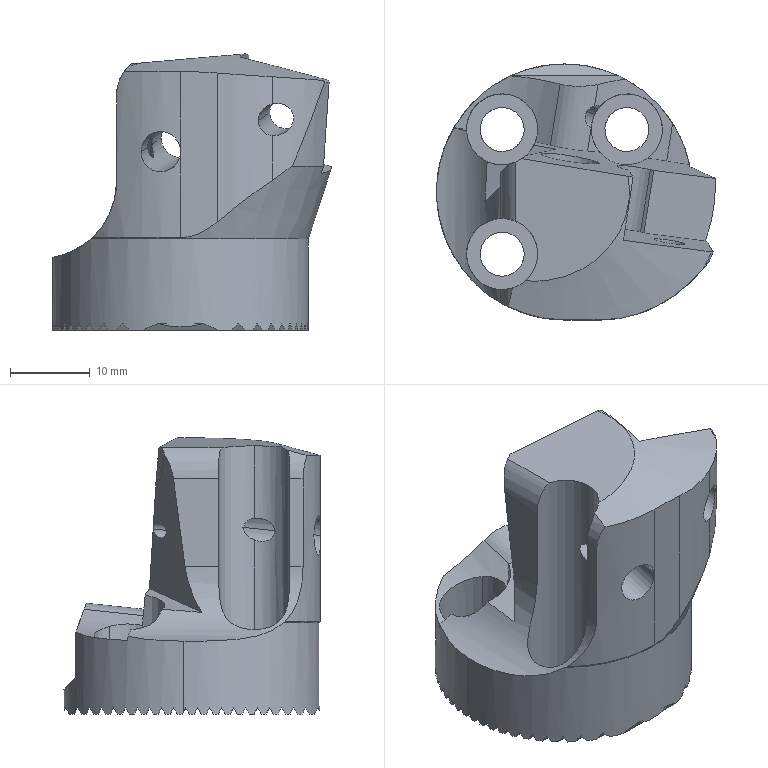NC program | Mastercam | posted with a generic post
Lines 1 to 700 of 7888:
%
:0001()
(MATERIAL - ALUMINUM MM - 2024)
(T4|12 FEMR |H4|XY STOCK TO LEAVE - .15|Z STOCK TO LEAVE - 0.)
(T5|6 FEMR |H5|XY STOCK TO LEAVE - .1|Z STOCK TO LEAVE - .1)
(T6|4 FEMR |H6|D6|WEAR COMP|TOOL DIA. - 4.|XY STOCK TO LEAVE - .05|Z STOCK TO LEAVE - .1)
(T7|4 FEMF |H7|D7|WEAR COMP|TOOL DIA. - 4.|XY STOCK TO LEAVE - 0.|Z STOCK TO LEAVE - .02)
(T9|12 FEMF |H9|D9|WEAR COMP|TOOL DIA. - 12.)
(T10|30 BNOS |H10|D10|WEAR COMP|TOOL DIA. - 30.)
(T12|6 SPD |H12)
(T3|4.3 DR |H3)
(T13|3.3 DR |H13)
(T1|2 DR |H1)
(T11|4 FEM |H11)
(T18|5.5 FL |H18)
(T14|3.15 THML |H14|D14|WEAR COMP|TOOL DIA. - 3.15)
(T16|M5 X 0.8 RH |H16)
(T15|2.5 BM |H15)
(T2|6 120DSPD |H2)
(T17|3 DR |H17)
N100 G21
N102 G0 G17 G40 G80 G90 G94 G98
N104 G0 G28 G91 Z0.
N106 G0 G28 X0. Y0.
(12 FEMR |TOOL - 4|DIA. OFF. - 4|LEN. - 4|TOOL DIA. - 12.)
N108 T4 M6
N110 G0 G54 G90 X25.327 Y-16.016 C0. B0. S3500 M3
N112 G43 H4 Z84.532
N114 Z36.532
N116 G1 Z9.782 F2000.
N118 X24.063 Y-14.854 Z9.631 F2500.
N120 G3 X23.099 Y-14.284 Z9.532 I-1.827 J-1.988
N122 X22.513 Y-14.091 I-2.505 J-6.624
N124 X22.076 Y-14.542 I1.447 J-1.839
N126 X20.527 Y-16.382 I63.197 J-54.78
N128 G2 X15.136 Y-21.366 I-22.56 J18.993
N130 X4.096 Y-25.849 I-15.051 J21.233
N132 X1.821 Y-25.988 I-2.275 J18.516
N134 X-.909 Y-25.787 J18.655
N136 X-14.128 Y-19.713 I3.68 J25.432
N138 X-21.534 Y-8.928 I17.053 J19.644
N140 G1 X-21.941
N142 X-22.348
N144 G3 X-23.443 Y-9.16 Z9.606 J-2.7
N146 G1 X-25.013 Y-9.857 Z9.72
N148 G3 X-25.778 Y-10.368 Z9.782 I1.096 J-2.467
N150 X-26.617 Y-12.324 I1.861 J-1.956
N152 X-24.238 Y-15.005 I2.7
N154 G2 X-19.964 Y-15.517 I-24.723 J-224.737 F9500.
N156 X-18.544 Y-16.345 I-.297 J-2.139
N158 G3 X-4.251 Y-26.044 I21.482 J16.278
N160 X2.015 Y-26.912 I6.266 J22.19
N162 X2.462 Y-26.907 J23.058
N164 X6.706 Y-26.267 I-.54 J17.966
N166 X17.663 Y-20.587 I-6.831 J26.583
N168 G2 X18.923 Y-20.181 I1.26 J-1.754
N170 X19.179 Y-20.196 J-2.16
N172 G1 X23.134 Y-20.669
N174 G3 X23.454 Y-20.688 I.32 J2.681
N176 X26.154 Y-17.988 J2.7
N178 X25.843 Y-16.729 I-2.7
N180 X25.281 Y-16. Z9.72 I-2.389 J-1.259 F2500.
N182 G1 X24.017 Y-14.838 Z9.606
N184 G3 X23.053 Y-14.268 Z9.532 I-1.827 J-1.988
N186 X22.433 Y-14.074 I-1.233 J-2.856
N188 X21.719 Y-14.71 I2.987 J-4.073
N190 X19.861 Y-16.692 I53.778 J-52.268
N192 G2 X15.195 Y-20.861 I-23.789 J21.932
N194 X5.469 Y-25.196 I-15.123 J20.849
N196 X1.763 Y-25.549 I-3.706 J19.282
N198 X-1.087 Y-25.341 J19.635
N200 X-11.914 Y-20.963 I3.638 J24.572
N202 X-20.634 Y-10.181 I14.952 J21.008
N204 G3 X-21.069 Y-9.298 I-25.07 J-11.815
N206 X-21.342 Y-8.928 I-1.084 J-.514
N208 G1 X-21.749
N210 G3 X-22.845 Y-9.16 Z9.606 J-2.7
N212 G1 X-24.414 Y-9.857 Z9.72
N214 G3 X-25.179 Y-10.368 Z9.782 I1.095 J-2.467
N216 X-26.018 Y-12.324 I1.86 J-1.956 F9500.
N218 X-23.642 Y-15.005 I2.699
N220 G2 X-19.481 Y-15.507 I-24.132 J-217.33
N222 X-18.075 Y-16.322 I-.3 J-2.14
N224 G3 X-3.802 Y-25.748 I20.927 J16.168
N226 X1.808 Y-26.475 I5.61 J21.278
N228 X3.413 Y-26.416 J22.005
N230 X8.741 Y-25.253 I-1.778 J20.92
N232 X17.208 Y-20.488 I-9.096 J26.07
N234 G2 X18.445 Y-20.099 I1.237 J-1.771
N236 X18.704 Y-20.114 J-2.16
N238 G1 X23.036 Y-20.637
N240 G3 X23.36 Y-20.657 I.324 J2.68
N242 X26.06 Y-17.957 J2.7
N244 X25.748 Y-16.697 I-2.7
N246 X25.187 Y-15.968 Z9.72 I-2.388 J-1.26 F2500.
N248 G1 X23.922 Y-14.807 Z9.606
N250 G3 X22.959 Y-14.236 Z9.532 I-1.827 J-1.988
N252 X22.374 Y-14.066 I-1.101 J-2.683
N254 X22.313 Y-14.06 I-.144 J-1.191
N256 X21.573 Y-14.633 I2.623 J-4.149
N258 X19.45 Y-16.705 I41.164 J-44.288
N260 G2 X15.167 Y-20.423 I-25.523 J25.078
N262 X6.987 Y-24.419 I-15.258 J20.865
N264 X1.726 Y-25.122 I-5.261 J19.345
N266 X-1.631 Y-24.838 J20.048
N268 X-12.379 Y-20.136 I4.116 J24.041
N270 X-19.695 Y-11.291 I15.466 J20.24
N272 G3 X-20.718 Y-9.43 I-20.626 J-10.132
N274 X-21.323 Y-8.928 I-1.027 J-.621
N276 G1 X-21.556 Y-9.857 Z9.595
N278 G3 X-21.752 Y-11.447 Z9.702 I6.34 J-1.59
N280 X-21.642 Y-12.646 Z9.782 I6.536
N282 X-18.925 Y-16.829 I6.426 J1.199 F9500.
N284 G1 X-7.24 Y-24.879
N286 G3 X-5.367 Y-25.77 I3.708 J5.382
N288 X1.244 Y-26.717 I6.611 J22.596
N290 X13.879 Y-23.04 J23.543
N292 G1 X24.283 Y-16.423
N294 X25.063 Y-15.927 Z9.72 F2500.
N296 X23.798 Y-14.765 Z9.606
N298 G3 X22.834 Y-14.194 Z9.532 I-1.827 J-1.988
N300 X22.21 Y-14.058 I-.624 J-1.364
N302 X22.151 Y-14.06 J-1.5
N304 X21.17 Y-14.768 I2.987 J-5.17
N306 X18.98 Y-16.767 I38.187 J-44.029
N308 G2 X14.652 Y-20.34 I-26.402 J27.573
N310 X7.861 Y-23.741 I-14.905 J21.276
N312 X1.707 Y-24.696 I-6.154 J19.347
N314 X-2.293 Y-24.299 J20.302
N316 X-13.296 Y-18.888 I4.768 J23.585
N318 X-18.729 Y-12.278 I16.488 J19.093
N320 G3 X-20.042 Y-10.033 I-75.514 J-42.648
N322 X-20.484 Y-9.389 I-27.464 J-18.386
N324 X-21.11 Y-8.928 I-.987 J-.683
N326 G1 X-21.305 Y-9.857 Z9.595
N328 G3 X-21.44 Y-11.156 Z9.682 I6.166 J-1.299
N330 X-21.26 Y-12.653 Z9.782 I6.301
N332 X-18.83 Y-16.264 I6.121 J1.497 F9500.
N334 G1 X-7.75 Y-24.269
N336 G3 X-6.03 Y-25.147 I3.69 J5.108
N338 X1.57 Y-26.366 I7.6 J23.09
N340 X13.907 Y-23.002 J24.309
N342 G1 X24.732 Y-16.625
N344 X24.828 Y-16.569 Z9.774 F2500.
N346 G3 X25.043 Y-16.193 Z9.744 I-.221 J.376
N348 X24.902 Y-15.872 Z9.72 I-.436
N350 G1 X23.638 Y-14.711 Z9.606
N352 G3 X22.674 Y-14.14 Z9.532 I-1.827 J-1.988
N354 X22.232 Y-14.057 I-.442 J-1.136
N356 X21.896 Y-14.104 J-1.219
N358 X21.255 Y-14.545 I1.025 J-2.182
N360 G2 X17.18 Y-18.101 I-18.947 J17.598
N362 G3 X16.536 Y-18.58 I237.78 J-319.951
N364 G2 X12.22 Y-21.428 I-22.586 J29.54
N366 X6.428 Y-23.721 I-11.391 J20.308
N368 X1.693 Y-24.279 I-4.735 J19.815
N370 X-3.706 Y-23.55 J20.373
N372 X-15.397 Y-16.261 I6.303 J23.129
N374 X-16.881 Y-14.418 I20.422 J17.958
N376 X-19.755 Y-10.15 I17.443 J14.849
N378 G3 X-20.293 Y-9.363 I-6.125 J-3.611
N380 X-20.812 Y-8.962 I-.966 J-.712
N382 X-21.095 Y-8.928 I-.283 J-1.166
N384 X-23.066 Y-9.783 Z9.678 J-2.7
N386 G1 X-23.649 Y-10.406 Z9.735
N388 G3 X-24.059 Y-10.979 Z9.782 I1.971 J-1.845
N390 X-24.377 Y-12.251 I2.381 J-1.272 F9500.
N392 X-21.678 Y-14.95 I2.699
N394 X-19.961 Y-14.335 J2.699
N396 X-18.978 Y-12.251 Z9.624 I-1.717 J2.084 F2500.
N398 X-19.327 Y-10.922 Z9.532 I-2.7
N400 G2 X-20.048 Y-9.556 I19.393 J11.113
N402 G3 X-20.789 Y-8.971 I-1.081 J-.607
N404 X-21.11 Y-8.927 Z9.553 I-.321 J-1.157
N406 X-22.169 Y-9.563 Z9.639 J-1.201
N408 G1 X-22.503 Y-10.189 Z9.686
N410 G3 X-22.689 Y-10.931 Z9.738 I1.39 J-.742
N412 X-22.55 Y-11.577 Z9.782 I1.576
N414 X-21.646 Y-12.413 I1.437 J.646 F9500.
N416 X-21.113 Y-12.506 Z9.746 I.533 J1.482 F2500.
N418 X-19.538 Y-10.931 Z9.582 J1.575
N420 X-19.715 Y-10.207 Z9.532 I-1.575
N422 G2 X-20.013 Y-9.608 I19.715 J10.207
N424 G3 X-21.095 Y-8.928 I-1.082 J-.52
N426 X-22.19 Y-9.16 Z9.606 J-2.7
N428 G1 X-23.76 Y-9.857 Z9.72
N430 G3 X-24.525 Y-10.368 Z9.782 I1.096 J-2.467
N432 X-25.364 Y-12.324 I1.861 J-1.956 F9500.
N434 X-23.093 Y-14.99 I2.7
N436 G1 X-17.635 Y-15.868
N438 G2 X-16.345 Y-16.586 I-.342 J-2.132
N440 G3 X-3.918 Y-24.455 I18.925 J16.14
N442 X1.691 Y-25.206 I5.609 J20.576
N444 X7.761 Y-24.324 J21.327
N446 X14.009 Y-21.457 I-7.621 J24.852
N448 G2 X15.106 Y-21.158 I1.097 J-1.861
N450 X15.448 Y-21.185 J-2.16
N452 G1 X20.574 Y-22.009
N454 G3 X21.002 Y-22.043 I.428 J2.666
N456 X23.702 Y-19.343 J2.7
N458 X21.574 Y-16.704 I-2.7
N460 X21.002 Y-16.643 Z9.744 I-.572 J-2.639 F2500.
N462 X20.386 Y-16.714 Z9.702 J-2.7
N464 G1 X20.385
N466 X18.98 Y-17.044 Z9.606
N468 G3 X17.966 Y-17.52 Z9.532 I.617 J-2.629
N470 G2 X14.756 Y-19.601 I-16.018 J21.202
N472 X11.208 Y-21.561 I-26.515 J43.803
N474 X5.266 Y-23.543 I-10.01 J20.109
N476 X1.705 Y-23.853 I-3.561 J20.299
N478 X-4.833 Y-22.789 J20.609
N480 X-13.656 Y-17.503 I7.425 J22.401
N482 X-17.147 Y-14.101 I13.656 J17.503
N484 G3 X-18.022 Y-13.402 Z9.606 I-2.085 J-1.715
N486 G1 X-19.285 Y-12.769 Z9.7
N488 G3 X-19.883 Y-12.628 Z9.741 I-.598 J-1.193
N490 X-20.471 Y-12.764 Z9.782 J-1.334
N492 X-21.107 Y-13.428 I.588 J-1.198 F9500.
N494 G1 X-22.287 Y-16.133
N496 G3 X-22.398 Y-16.667 I1.224 J-.534
N498 X-21.614 Y-17.883 I1.335
N500 G1 X-14.889 Y-20.925
N502 G3 X6.013 Y-25.433 I20.902 J46.199
N504 X14.41 Y-24.733 J50.707
N506 G1 X19.513 Y-23.877
N508 G3 X21.779 Y-21.199 I-.449 J2.678
N510 X19.291 Y-18.493 I-2.715
N512 X19.064 Y-18.483 Z9.767 I-.227 J-2.706 F2500.
N514 X18.743 Y-18.503 Z9.745 J-2.716
N516 G1 X18.098 Y-18.579 Z9.702
N518 X16.664 Y-18.75 Z9.606
N520 G3 X15.604 Y-19.11 Z9.532 I.319 J-2.681
N522 G2 X12.148 Y-20.826 I-13.308 J22.47
N524 X8.231 Y-22.392 I-15.934 J34.155
N526 X1.744 Y-23.434 I-6.487 J19.662
N528 X-5.935 Y-21.958 J20.704
N530 X-10.399 Y-19.614 I8.614 J21.825
N532 X-14.116 Y-17.134 I10.399 J19.614
N534 G3 X-15.11 Y-16.616 Z9.606 I-1.717 J-2.084
N536 G1 X-16.471 Y-16.238 Z9.7
N538 G3 X-16.829 Y-16.189 Z9.724 I-.358 J-1.287
N540 X-17.636 Y-16.46 Z9.782 J-1.336
N542 X-18.061 Y-17.008 I.807 J-1.065 F9500.
N544 G1 X-19.203 Y-19.731
N546 G3 X-19.307 Y-20.248 I1.233 J-.517
N548 X-18.313 Y-21.539 I1.337
N550 X12.208 Y-25.517 I30.521 J115.1
N552 X17.041 Y-25.419 J119.078
N554 X19.638 Y-22.714 I-.11 J2.705
N556 X17.119 Y-20.013 I-2.707
N558 X16.931 Y-20.006 Z9.769 I-.188 J-2.701 F2500.
N560 G1 X16.9 Y-20.007 Z9.767
N562 X15.891 Y-20.019 Z9.7
N564 X14.477 Y-20.035 Z9.606
N566 G3 X13.385 Y-20.28 Z9.532 I.032 J-2.7
N568 G2 X10.176 Y-21.457 I-9.354 J20.546
N570 X6.628 Y-22.471 I-12.999 J38.767
N572 X1.85 Y-23.021 I-4.778 J20.468
N574 X-6.993 Y-21.07 J21.018
N576 X-10.717 Y-19.442 I6.993 J21.07
N578 G3 X-12.02 Y-19.107 Z9.622 I-1.303 J-2.365
N580 X-14.122 Y-20.113 Z9.782 J-2.7
N582 X-14.72 Y-21.807 I2.102 J-1.694 F9500.
N584 X-12.236 Y-24.498 I2.7
N586 G1 X11.728 Y-26.426
N588 G3 X11.945 Y-26.435 I.217 J2.692
N590 X14.646 Y-23.734 J2.701
N592 X14.329 Y-22.467 I-2.701
N594 X11.945 Y-21.034 Z9.588 I-2.384 J-1.267 F2500.
N596 X11.111 Y-21.166 Z9.532 J-2.7
N598 G2 X7.78 Y-21.965 I-6.85 J21.232
N600 X4.086 Y-22.527 I-7.479 J36.716
N602 X2.041 Y-22.624 I-2.045 J21.433
N604 X-3.282 Y-21.956 J21.53
N606 X-7.613 Y-20.854 I3.282 J21.956
N608 G3 X-8.539 Y-20.69 Z9.595 I-.926 J-2.536
N610 X-10.876 Y-22.038 Z9.782 J-2.7
N612 X-11.239 Y-23.39 I2.337 J-1.352 F9500.
N614 X-8.696 Y-26.086 I2.7
N616 G1 X9.125 Y-27.127
N618 G3 X9.282 Y-27.132 I.157 J2.695
N620 X11.982 Y-24.432 J2.7
N622 X11.797 Y-23.448 I-2.7
N624 X9.282 Y-21.731 Z9.568 I-2.515 J-.984 F2500.
N626 X8.75 Y-21.785 Z9.532 J-2.701
N628 G2 X4.925 Y-22.206 I-4.342 J21.859
N630 X2.83 Y-22.274 I-2.095 J32.189
N632 X.646 Y-22.2 J32.257
N634 G1 X.239
N636 G2 X.021 Y-22.201 I-.218 J22.375
N638 X-3.646 Y-21.899 J22.376
N640 G3 X-4.09 Y-21.862 Z9.562 I-.444 J-2.663
N642 X-6.635 Y-23.663 Z9.782 J-2.7
N644 X-6.789 Y-24.562 I2.545 J-.899 F9500.
N646 X-4.166 Y-27.261 I2.699
N648 G1 X6.023 Y-27.55
N650 G3 X6.1 Y-27.551 I.077 J2.698
N652 X8.799 Y-24.852 J2.699
N654 X8.723 Y-24.214 I-2.699
N656 X6.1 Y-22.153 Z9.543 I-2.623 J-.638 F2500.
N658 X5.928 Y-22.157 Z9.532 J-2.699
N660 G2 X4.074 Y-22.208 I-1.854 J33.96
N662 X3.359 Y-22.2 J34.011
N664 G1 X2.952
N666 X0.
N668 G3 X-1.096 Y-22.432 Z9.606 J-2.7
N670 G1 X-2.387 Y-23.006 Z9.7
N672 G3 X-3.36 Y-23.738 Z9.782 I1.096 J-2.467
N674 X-3.991 Y-25.473 I2.069 J-1.735 F9500.
N676 X-1.291 Y-28.173 I2.7
N678 X-.435 Y-28.034 J2.7
N680 G1 X23.234 Y-20.118
N682 G3 X25.077 Y-17.558 I-.856 J2.56
N684 G1 X25.063 Y-17.283
N686 X25.021 Y-17.011
N688 X24.952 Y-16.744
N690 G3 X24.312 Y-15.673 Z9.698 I-2.575 J-.814 F2500.
N692 G1 X23.089 Y-14.419 Z9.582
N694 G3 X22.428 Y-14.073 Z9.532 I-.859 J-.838
N696 X22.23 Y-14.057 I-.198 J-1.184
N698 X21.346 Y-14.446 J-1.2
N700 G2 X20.786 Y-15.036 I-18.731 J17.193
N702 G3 X20.186 Y-15.982 Z9.641 I1.93 J-1.889
N704 G1 X19.682 Y-17.335 Z9.782
N706 G0 Z84.532
N708 C9. B-84.
N710 X13.169 Y27.825
N712 Z56.789
N714 Z8.789
N716 G1 Z7.039 F2000.
N718 X12.949 Y26.122 Z6.888 F2500.
N720 G3 X12.927 Y25.777 Z6.858 I2.678 J-.345
N722 X13.04 Y25.006 Z6.789 I2.7
N724 G1 X13.214 Y24.421
N726 X13.479 Y24.43
N728 G3 X15.936 Y24.972 I-3.086 J19.807
N730 X19.38 Y25.938 I-41.706 J155.352
N732 G2 X22.887 Y26.414 I4.411 J-19.32
N734 X27.937 Y26.532 I5.05 J-108.202
N736 X28.468 Y26.531 J-108.32
N738 X30.923 Y26.536 I3.173 J-965.361
N740 G1 X31.331
N742 X34.477
N744 G2 X37.69 Y25.537 I-.189 J-6.275
N746 X40.163 Y22.946 I-4.167 J-6.454
N748 X41.389 Y19.73 I-9.311 J-5.391
N750 X41.824 Y16.067 I-21.737 J-4.435
N752 X41.922 Y10.577 I-154.13 J-5.49
N754 X41.919 Y9.72 I-154.228
N756 G1 X41.92 Y9.311
N758 X41.913 Y-16.351
N760 G2 X40.808 Y-19.535 I-6.329 J.413
N762 X38.186 Y-21.918 I-6.343 J4.345
N764 X34.999 Y-23.084 I-5.317 J9.594
N766 X31.365 Y-23.498 I-4.394 J22.434
N768 X25.885 Y-23.592 I-5.48 J160.417
N770 X25.027 Y-23.589 J160.511
N772 G1 X24.618
N774 X15.311 Y-23.592
N776 Y-24.406
N778 G3 X15.543 Y-25.502 Z6.863 I2.7
N780 G1 X16.24 Y-27.071 Z6.977
N782 G3 X16.692 Y-27.877 Z7.039 I4.547 J2.019
N784 X20.787 Y-30.027 I4.095 J2.825
N786 X22.619 Y-29.678 J4.975
N788 G1 X39.035 Y-23.18 F9500.
N790 G3 X43.527 Y-16.596 I-2.616 J6.609
N792 G1 X43.649 Y17.94
N794 Y17.979
N796 G3 X32.572 Y29.056 I-11.077
N798 X31.838 Y29.031 J-11.077
N800 G1 X14.101 Y27.854
N802 X13.179 Y27.792 Z6.977 F2500.
N804 X12.959 Y26.089 Z6.863
N806 G3 X12.937 Y25.744 Z6.84 I2.678 J-.345
N808 X13.049 Y24.973 Z6.789 I2.7
N810 G1 X13.224 Y24.388
N812 X13.231 Y24.364
N814 G3 X13.544 Y24.347 I.313 J2.895
N816 X13.98 Y24.38 J2.912
N818 X16.814 Y24.953 I-2.564 J20.002
N820 X17.567 Y25.15 I-23.076 J89.671
N822 G2 X23.806 Y26.1 I7.402 J-27.64
N824 X29.697 Y26.23 I5.891 J-133.363
N826 X30.173 Y26.229 J-133.493
N828 X31.45 Y26.233 I1.277 J-224.484
N830 X32.81 Y26.229 J-224.488
N832 X38.496 Y23.57 I-.274 J-7.995
N834 X40.634 Y19.8 I-7.655 J-6.833
N836 X41.369 Y16.142 I-16.439 J-5.203
N838 X41.595 Y11.208 I-56.097 J-5.039
N840 X41.625 Y3.67 I-962.807 J-7.538
N842 X41.622 Y1.78 I-962.837
N844 G1 Y1.373
N846 X41.616 Y-14.483
N848 G2 X38.958 Y-20.164 I-7.998 J.279
N850 X35.185 Y-22.304 I-6.835 J7.655
N852 X31.528 Y-23.038 I-5.203 J16.443
N854 X26.594 Y-23.264 I-5.04 J56.104
N856 X18.342 Y-23.299 I-8.252 J962.918
N858 X16.494 Y-23.298 J962.953
N860 G3 X15.311 Y-23.4 I.481 J-12.422
N862 G1 Y-23.807
N864 Y-24.214
N866 G3 X15.543 Y-25.31 Z6.863 I2.7
N868 G1 X16.24 Y-26.879 Z6.977
N870 G3 X16.692 Y-27.685 Z7.039 I4.521 J2.007
N872 X20.761 Y-29.819 I4.069 J2.813 F9500.
N874 X22.695 Y-29.425 J4.947
N876 G1 X38.839 Y-22.567
N878 G3 X43.142 Y-16.141 I-2.763 J6.504
N880 G1 X43.498 Y16.192
N882 G3 X43.499 Y16.32 I-11.709 J.128
N884 X32.628 Y27.999 I-11.71
N886 G1 X14.95 Y29.269
N888 G3 X14.833 Y29.273 I-.117 J-1.628
N890 X13.504 Y28.589 J-1.632
N892 X13.213 Y27.849 Z6.985 I1.329 J-.948 F2500.
N894 G1 X13.198 Y27.729 Z6.977
N896 X12.978 Y26.026 Z6.863
N898 G3 X12.956 Y25.68 Z6.84 I2.678 J-.346
N900 X13.068 Y24.909 Z6.789 I2.7
N902 G1 X13.243 Y24.324
N904 X13.252 Y24.293
N906 G3 X13.771 Y24.248 I.519 J2.991
N908 X13.989 Y24.256 J3.036
N910 X16.329 Y24.599 I-.878 J14.168
N912 G2 X20.203 Y25.372 I14.184 J-61.004
N914 X26.096 Y25.856 I6.84 J-47.128
N916 X30.163 Y25.916 I4.067 J-137.978
N918 X31.59 Y25.909 J-138.038
N920 X38.652 Y22.091 I-.298 J-8.992
N922 X40.356 Y18.556 I-9.664 J-6.837
N924 X41.059 Y14.8 I-18.914 J-5.484
N926 X41.293 Y9.478 I-64.709 J-5.518
N928 X41.323 Y1.839 I-959.204 J-7.639
N930 X41.322 Y.052 I-959.234
N932 G1 Y-.355
N934 X41.321 Y-12.61
N936 G2 X41.322 Y-12.744 I-9.97 J-.134
N938 X40.737 Y-16.11 I-9.971
N940 X37.22 Y-20.503 I-8.607 J3.286
N942 X33.422 Y-22.173 I-6.783 J10.272
N944 X29.288 Y-22.806 I-5.569 J22.553
N946 X23.764 Y-22.975 I-5.524 J90.019
N948 G1 X23.664
N950 G2 X17.624 Y-22.998 I-6.39 J876.896
N952 G3 X15.951 Y-23.11 I.09 J-13.927
N954 G2 X15.311 Y-23.224 I-3.931 J20.191
N956 G1 Y-23.631
N958 Y-24.038
N960 G3 X15.543 Y-25.134 Z6.863 I2.7
N962 G1 X16.24 Y-26.703 Z6.977
N964 G3 X16.692 Y-27.508 Z7.039 I4.51 J2.002
N966 X20.75 Y-29.635 I4.058 J2.807 F9500.
N968 X22.877 Y-29.153 J4.934
N970 G1 X38.611 Y-21.638
N972 G3 X42.54 Y-16.351 I-3.038 J6.36
N974 X42.695 Y-14.332 I-13.104 J2.019
N976 X42.693 Y-14.096 I-13.259
N978 G1 X42.116 Y18.27
N980 G3 X33.839 Y27.331 I-9.279 J-.166
N982 G1 X15.36 Y29.338
N984 G3 X15.15 Y29.349 I-.21 J-1.934
N986 X13.548 Y28.508 J-1.945
N988 X13.22 Y27.652 Z6.977 I1.602 J-1.104 F2500.
N990 G1 X13.001 Y25.949 Z6.863
N992 G3 X12.979 Y25.604 Z6.84 I2.678 J-.345
N994 X13.091 Y24.833 Z6.789 I2.7
N996 G1 X13.266 Y24.248
N998 X13.276 Y24.213
N1000 G3 X13.948 Y24.134 I.672 J2.807
N1002 G1 X13.999
N1004 G3 X16.275 Y24.364 I-.096 J12.333
N1006 G2 X20.45 Y25.071 I19.385 J-101.678
N1008 X27.097 Y25.56 I7.674 J-58.939
N1010 X29.189 Y25.597 I2.092 J-59.845
N1012 X30.556 Y25.581 J-59.882
N1014 X34.786 Y24.475 I-.4 J-10.17
N1016 X38.801 Y20.549 I-4.713 J-8.837
N1018 X40.218 Y16.932 I-11.919 J-6.754
N1020 X40.817 Y12.882 I-24.53 J-5.7
N1022 X41.004 Y6.886 I-96.191 J-5.996
N1024 G1 Y6.841
N1026 G2 X41.021 Y1.163 I-932.762 J-5.678
N1028 G1 Y.699
N1030 Y.291
N1032 X41.014 Y-11.635
N1034 G2 X40.415 Y-15.212 I-11.392 J.068
N1036 X36.634 Y-20.037 I-9.205 J3.319
N1038 X32.946 Y-21.722 I-7.087 J10.638
N1040 X28.792 Y-22.444 I-5.917 J21.712
N1042 X23.106 Y-22.666 I-5.783 J75.422
N1044 X18.658 Y-22.696 I-5.769 J516.961
N1046 G1 X18.612
N1048 G3 X16.161 Y-22.863 J-18.02
N1050 X15.311 Y-23.055 I1.337 J-7.897
N1052 G1 Y-23.462
N1054 Y-23.869
N1056 G3 X15.543 Y-24.965 Z6.863 I2.7
N1058 G1 X16.24 Y-26.534 Z6.977
N1060 G3 X16.692 Y-27.34 Z7.039 I4.527 J2.009
N1062 X20.767 Y-29.478 I4.075 J2.815 F9500.
N1064 X23.057 Y-28.917 J4.953
N1066 G1 X38.582 Y-20.823
N1068 G3 X42.384 Y-14.723 I-3.271 J6.274
N1070 G1 X43.074 Y13.261
N1072 G3 X43.078 Y13.603 I-13.882 J.342
N1074 X30.865 Y27.388 I-13.886
N1076 G1 X15.423 Y29.262
N1078 G3 X15.187 Y29.276 I-.236 J-1.943
N1080 X13.572 Y28.425 J-1.957
N1082 X13.245 Y27.569 Z6.977 I1.615 J-1.106 F2500.
N1084 G1 X13.026 Y25.866 Z6.863
N1086 G3 X13.004 Y25.521 Z6.84 I2.678 J-.345
N1088 X13.116 Y24.75 Z6.789 I2.7
N1090 G1 X13.29 Y24.165
N1092 X13.302 Y24.126
N1094 G3 X14.01 Y24.012 I.79 J2.651
N1096 X14.466 Y24.003 I.456 J11.585
N1098 X16.242 Y24.14 J11.594
N1100 X19.398 Y24.606 I-16.281 J121.076
N1102 G2 X27.708 Y25.256 I9.416 J-66.991
N1104 X28.533 Y25.273 I.825 J-19.828
N1106 X30.421 Y25.183 J-19.845
N1108 X38.146 Y20.362 I-.979 J-10.168
N1110 X39.858 Y16.238 I-11.765 J-7.302
N1112 X40.518 Y11.748 I-25.54 J-6.045
N1114 X40.702 Y5.729 I-101.471 J-6.111
N1116 X40.722 Y-.542 I-984.598 J-6.271
N1118 X40.721 Y-1.23 I-984.618
N1120 G1 Y-1.638
N1122 X40.716 Y-10.263
N1124 Y-10.312
N1126 G2 X40.392 Y-13.357 I-14.479
N1128 X35.952 Y-19.692 I-9.996 J2.282
N1130 X32.086 Y-21.408 I-7.344 J11.333
N1132 X27.991 Y-22.118 I-6.067 J22.844
N1134 X22.297 Y-22.359 I-5.955 J73.239
N1136 X19.86 Y-22.385 I-9.834 J798.387
N1138 G1 X19.827
N1140 G3 X16.828 Y-22.547 J-27.865
N1142 X15.311 Y-22.89 I.804 J-7.075
N1144 G1 Y-23.297
N1146 Y-23.704
N1148 G3 X15.543 Y-24.8 Z6.863 I2.7
N1150 G1 X16.24 Y-26.369 Z6.977
N1152 G3 X16.692 Y-27.174 Z7.039 I4.517 J2.005
N1154 X20.757 Y-29.306 I4.065 J2.81 F9500.
N1156 X23.201 Y-28.66 J4.942
N1158 G1 X38.334 Y-20.052
N1160 G3 X41.844 Y-14.831 I-3.491 J6.137
N1162 X41.951 Y-13.184 I-12.588 J1.647
N1164 G1 Y-13.068
N1166 X41.699 Y14.399
N1168 G3 X31.375 Y26.754 I-12.694 J-.116
N1170 G1 X16.238 Y29.632
N1172 G3 X15.768 Y29.676 I-.47 J-2.473
N1174 X13.554 Y28.355 J-2.517
N1176 X13.272 Y27.48 Z6.977 I2.214 J-1.196 F2500.
N1178 G1 X13.052 Y25.777 Z6.863
N1180 G3 X13.03 Y25.432 Z6.84 I2.678 J-.345
N1182 X13.142 Y24.661 Z6.789 I2.7
N1184 G1 X13.317 Y24.076
N1186 X13.329 Y24.035
N1188 G3 X14.024 Y23.89 I.894 J2.547
N1190 X14.95 Y23.851 I.926 J11.01
N1192 X16.217 Y23.924 J11.049
N1194 X20.117 Y24.397 I-13.82 J130.316
N1196 G2 X28.09 Y24.923 I8.699 J-71.227
N1198 G1 X28.127
N1200 G2 X31.673 Y24.443 J-13.351
N1202 X37.501 Y20.183 I-2.968 J-10.177
N1204 X39.287 Y16.378 I-11.401 J-7.674
N1206 X40.131 Y11.784 I-22.512 J-6.51
N1208 X40.383 Y6.091 I-73.221 J-6.098
N1210 X40.424 Y-2.868 I-982.271 J-8.959
N1212 X40.422 Y-4.972 I-982.312
N1214 G1 Y-5.379
N1216 G2 X40.424 Y-6.426 I-286.016 J-1.047
N1218 X40.406 Y-9.585 I-286.018
N1220 X39.987 Y-12.945 I-14.559 J.11
N1222 X35.38 Y-19.312 I-10.376 J2.658
N1224 X31.321 Y-21.089 I-7.634 J11.913
N1226 X26.801 Y-21.835 I-6.357 J24.461
N1228 X21.175 Y-22.061 I-6.177 J83.607
N1230 G3 X17.562 Y-22.221 I.104 J-43.147
N1232 X15.843 Y-22.542 I.943 J-9.822
N1234 G2 X15.311 Y-22.728 I-8.82 J24.391
N1236 G1 Y-23.135
N1238 Y-23.542
N1240 G3 X15.543 Y-24.637 Z6.863 I2.7
N1242 G1 X16.24 Y-26.207 Z6.977
N1244 G3 X16.692 Y-27.012 Z7.039 I4.548 J2.019
N1246 X20.788 Y-29.163 I4.096 J2.824 F9500.
N1248 X23.435 Y-28.401 J4.975
N1250 G1 X38.226 Y-19.107
N1252 G3 X41.436 Y-14.366 I-3.782 J6.018
N1254 X41.634 Y-12.351 I-11.976 J2.188
N1256 G1 X42.008 Y14.008
N1258 G3 X42.009 Y14.181 I-12.173 J.173
N1260 X32.362 Y26.09 I-12.174
N1262 G1 X16.281 Y29.502
N1264 G3 X15.765 Y29.556 I-.516 J-2.432
N1266 X13.583 Y28.262 J-2.486
N1268 X13.299 Y27.388 Z6.977 I2.182 J-1.192 F2500.
N1270 G1 X13.08 Y25.685 Z6.863
N1272 G3 X13.058 Y25.34 Z6.84 I2.678 J-.345
N1274 X13.17 Y24.569 Z6.789 I2.7
N1276 G1 X13.344 Y23.984
N1278 X13.357 Y23.94
N1280 G3 X14.043 Y23.767 I.992 J2.482
N1282 X15.379 Y23.684 I1.336 J10.718
N1284 X16.2 Y23.716 J10.801
N1286 X19.99 Y24.085 I-6.241 J83.694
N1288 G2 X26.514 Y24.565 I9.467 J-84.072
N1290 X27.174 Y24.579 I.66 J-16.038
N1292 X30.022 Y24.324 J-16.052
N1294 X37.27 Y19.421 I-2.013 J-10.784
N1296 X39.114 Y15.151 I-12.306 J-7.851
N1298 X39.848 Y10.67 I-25.421 J-6.461
N1300 X40.088 Y4.598 I-86.108 J-6.448
N1302 X40.123 Y-3.708 I-996.654 J-8.306
N1304 X40.122 Y-5.232 I-996.689
N1306 G1 Y-5.64
N1308 G2 X40.125 Y-6.392 I-100.265 J-.752
N1310 X40.088 Y-9.113 I-100.268
N1312 X39.513 Y-12.801 I-14.506 J.373
N1314 X34.873 Y-18.917 I-10.627 J3.243
N1316 X30.61 Y-20.771 I-7.889 J12.315
N1318 X26.124 Y-21.513 I-6.486 J25.266
N1320 X20.956 Y-21.757 I-6.815 J89.515
N1322 G3 X17.764 Y-21.951 I.737 J-38.376
N1324 X15.811 Y-22.366 I.974 J-9.388
N1326 G2 X15.311 Y-22.566 I-8.668 J20.945
N1328 G1 Y-22.973
N1330 Y-23.38
N1332 G3 X15.543 Y-24.476 Z6.863 I2.7
N1334 G1 X16.24 Y-26.045 Z6.977
N1336 G3 X16.751 Y-26.81 Z7.039 I2.468 J1.095
N1338 X18.708 Y-27.65 I1.957 J1.86 F9500.
N1340 X21.408 Y-24.95 J2.7
N1342 X21.406 Y-24.846 I-2.7
N1344 G2 X21.404 Y-24.763 I2.159 J.083
N1346 X23.499 Y-22.604 I2.161
N1348 G3 X28.683 Y-22.132 I-1.221 J42.077
N1350 X33.528 Y-20.712 I-2.872 J18.777
N1352 X38.346 Y-17.006 I-5.213 J11.763
N1354 X40.85 Y-11.027 I-9.647 J7.554
N1356 X41.049 Y-7.969 I-23.429 J3.058
N1358 X41.047 Y-7.703 I-23.628
N1360 X41.05 Y-5.159 I-929.799 J2.544
N1362 G1 Y-4.01
N1364 Y-3.603
N1366 G3 X41.052 Y-2.055 I-520.916 J1.548
N1368 X40.978 Y6.736 I-520.918
N1370 X40.612 Y12.261 I-53.501 J-.773
N1372 X39.475 Y17.071 I-21.26 J-2.482
N1374 X36.522 Y21.845 I-12.825 J-4.634
N1376 X29.387 Y25.366 I-8.517 J-8.272
N1378 X27.015 Y25.506 I-2.372 J-20.071
N1380 X25.966 Y25.478 J-20.211
N1382 X21.068 Y25.13 I3.516 J-84.11
N1384 G2 X20.854 Y25.119 I-.214 J2.149
N1386 X18.699 Y27.132 J2.16
N1388 G3 X16.006 Y29.646 I-2.693 J-.185
N1390 X13.599 Y28.171 J-2.699
N1392 X13.328 Y27.292 Z6.977 I2.407 J-1.224 F2500.
N1394 G1 X13.108 Y25.589 Z6.863
N1396 G3 X13.086 Y25.244 Z6.84 I2.678 J-.345
N1398 X13.199 Y24.473 Z6.789 I2.7
N1400 G1 X13.373 Y23.888
N1402 X13.386 Y23.842
N1404 G3 X14.065 Y23.642 I1.089 J2.44
N1406 X15.758 Y23.503 I1.693 J10.255
N1408 X16.185 Y23.512 J10.394
N1410 X19.879 Y23.785 I-2.34 J56.756
N1412 G2 X25.46 Y24.198 I10.578 J-105.079
N1414 X26.393 Y24.222 I.933 J-17.974
N1416 X29.113 Y24.016 J-17.998
N1418 X36.855 Y18.965 I-1.745 J-11.135
N1420 X38.723 Y14.743 I-12.467 J-8.042
N1422 X39.507 Y10.255 I-24.948 J-6.665
N1424 X39.78 Y4.154 I-79.489 J-6.616
N1426 X39.819 Y-2.798 I-626.462 J-6.952
N1428 X39.798 Y-7.877 I-626.501
N1430 X39.427 Y-11.248 I-18.248 J.301
N1432 X34.125 Y-18.697 I-11.245 J2.392
N1434 X30.201 Y-20.382 I-7.885 J12.952
N1436 X25.713 Y-21.171 I-6.692 J24.881
N1438 X20.984 Y-21.449 I-7.476 J87.067
N1440 G3 X17.532 Y-21.742 I.87 J-30.699
N1442 X15.724 Y-22.22 I1.174 J-8.103
N1444 G1 X15.311 Y-22.406
N1446 Y-23.22
N1448 G3 X15.543 Y-24.316 Z6.863 I2.7
N1450 G1 X16.24 Y-25.885 Z6.977
N1452 G3 X16.689 Y-26.692 Z7.039 I4.724 J2.097
N1454 X20.964 Y-28.956 I4.275 J2.904 F9500.
N1456 X24.161 Y-27.849 J5.168